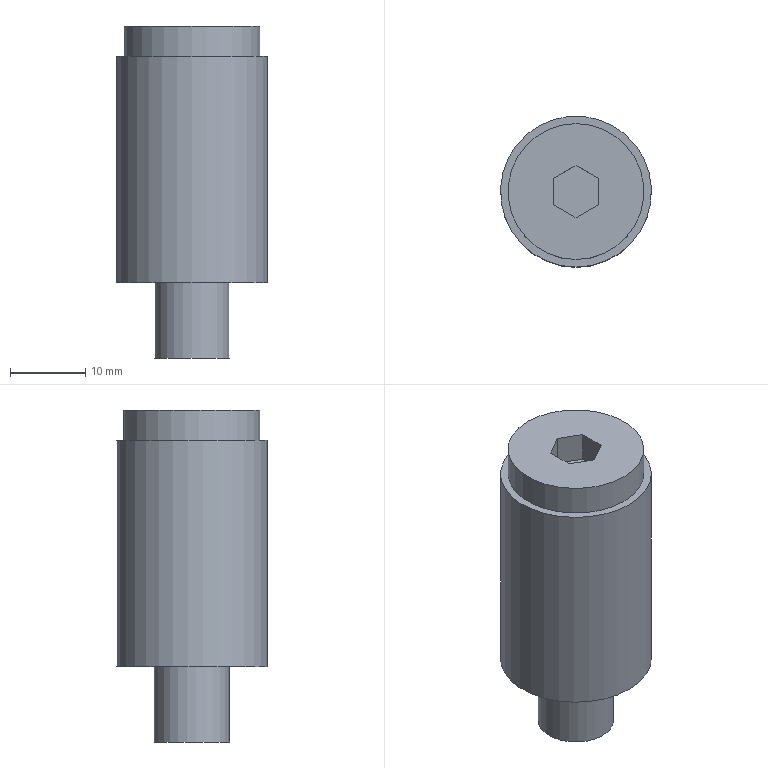Part | STEP file | 1_id570_xmt_txt | 1 solid | 17 faces | box 20 x 20 x 44 mm | volume 10770 mm3 | plane 12 | cylinder 4 | cone 1 | commonest cylinder face diameters 10 x1 11 x1 18 x1 20 x1
STEP:
#1=CARTESIAN_POINT('',(165.,186.,52.));
#2=VERTEX_POINT('',#1);
#3=CARTESIAN_POINT('',(165.,195.,52.));
#4=DIRECTION('',(0.,0.,1.));
#5=DIRECTION('',(0.,-1.,0.));
#6=AXIS2_PLACEMENT_3D('',#3,#4,#5);
#7=CIRCLE('',#6,9.);
#8=EDGE_CURVE('',#2,#2,#7,.T.);
#9=ORIENTED_EDGE('',*,*,#8,.F.);
#10=EDGE_LOOP('',(#9));
#11=FACE_BOUND('',#10,.T.);
#12=CARTESIAN_POINT('',(165.,186.,48.));
#13=VERTEX_POINT('',#12);
#14=CARTESIAN_POINT('',(165.,195.,48.));
#15=DIRECTION('',(0.,0.,-1.));
#16=DIRECTION('',(0.,-1.,0.));
#17=AXIS2_PLACEMENT_3D('',#14,#15,#16);
#18=CIRCLE('',#17,9.);
#19=EDGE_CURVE('',#13,#13,#18,.T.);
#20=ORIENTED_EDGE('',*,*,#19,.F.);
#21=EDGE_LOOP('',(#20));
#22=FACE_BOUND('',#21,.T.);
#23=CARTESIAN_POINT('',(165.,195.,50.));
#24=DIRECTION('',(0.,0.,-1.));
#25=DIRECTION('',(0.,1.,0.));
#26=AXIS2_PLACEMENT_3D('',#23,#24,#25);
#27=CYLINDRICAL_SURFACE('',#26,9.);
#28=ADVANCED_FACE('',(#11,#22),#27,.T.);
#29=CARTESIAN_POINT('',(165.,189.6,48.));
#30=VERTEX_POINT('',#29);
#31=CARTESIAN_POINT('',(165.,195.,48.));
#32=DIRECTION('',(0.,0.,1.));
#33=DIRECTION('',(0.,-1.,0.));
#34=AXIS2_PLACEMENT_3D('',#31,#32,#33);
#35=CIRCLE('',#34,5.4);
#36=EDGE_CURVE('',#30,#30,#35,.T.);
#37=ORIENTED_EDGE('',*,*,#36,.F.);
#38=EDGE_LOOP('',(#37));
#39=FACE_BOUND('',#38,.T.);
#40=CARTESIAN_POINT('',(165.,190.,23.));
#41=VERTEX_POINT('',#40);
#42=CARTESIAN_POINT('',(165.,195.,23.));
#43=DIRECTION('',(0.,0.,-1.));
#44=DIRECTION('',(0.,-1.,0.));
#45=AXIS2_PLACEMENT_3D('',#42,#43,#44);
#46=CIRCLE('',#45,5.);
#47=EDGE_CURVE('',#41,#41,#46,.T.);
#48=ORIENTED_EDGE('',*,*,#47,.F.);
#49=EDGE_LOOP('',(#48));
#50=FACE_BOUND('',#49,.T.);
#51=CARTESIAN_POINT('',(165.,195.,35.5));
#52=DIRECTION('',(0.,0.,1.));
#53=DIRECTION('',(0.,1.,0.));
#54=AXIS2_PLACEMENT_3D('',#51,#52,#53);
#55=CONICAL_SURFACE('',#54,5.2,0.9167);
#56=ADVANCED_FACE('',(#39,#50),#55,.T.);
#57=ORIENTED_EDGE('',*,*,#47,.T.);
#58=EDGE_LOOP('',(#57));
#59=FACE_BOUND('',#58,.T.);
#60=CARTESIAN_POINT('',(165.,190.,8.));
#61=VERTEX_POINT('',#60);
#62=CARTESIAN_POINT('',(165.,195.,8.));
#63=DIRECTION('',(0.,0.,-1.));
#64=DIRECTION('',(0.,-1.,0.));
#65=AXIS2_PLACEMENT_3D('',#62,#63,#64);
#66=CIRCLE('',#65,5.);
#67=EDGE_CURVE('',#61,#61,#66,.T.);
#68=ORIENTED_EDGE('',*,*,#67,.F.);
#69=EDGE_LOOP('',(#68));
#70=FACE_BOUND('',#69,.T.);
#71=CARTESIAN_POINT('',(165.,195.,15.5));
#72=DIRECTION('',(0.,0.,-1.));
#73=DIRECTION('',(0.,1.,0.));
#74=AXIS2_PLACEMENT_3D('',#71,#72,#73);
#75=CYLINDRICAL_SURFACE('',#74,5.);
#76=ADVANCED_FACE('',(#59,#70),#75,.T.);
#77=CARTESIAN_POINT('',(165.,185.,48.));
#78=VERTEX_POINT('',#77);
#79=CARTESIAN_POINT('',(165.,195.,48.));
#80=DIRECTION('',(0.,0.,1.));
#81=DIRECTION('',(0.,-1.,0.));
#82=AXIS2_PLACEMENT_3D('',#79,#80,#81);
#83=CIRCLE('',#82,10.);
#84=EDGE_CURVE('',#78,#78,#83,.T.);
#85=ORIENTED_EDGE('',*,*,#84,.F.);
#86=EDGE_LOOP('',(#85));
#87=FACE_BOUND('',#86,.T.);
#88=CARTESIAN_POINT('',(165.,185.,18.));
#89=VERTEX_POINT('',#88);
#90=CARTESIAN_POINT('',(165.,195.,18.));
#91=DIRECTION('',(0.,0.,-1.));
#92=DIRECTION('',(0.,-1.,0.));
#93=AXIS2_PLACEMENT_3D('',#90,#91,#92);
#94=CIRCLE('',#93,10.);
#95=EDGE_CURVE('',#89,#89,#94,.T.);
#96=ORIENTED_EDGE('',*,*,#95,.F.);
#97=EDGE_LOOP('',(#96));
#98=FACE_BOUND('',#97,.T.);
#99=CARTESIAN_POINT('',(165.,195.,33.));
#100=DIRECTION('',(0.,0.,-1.));
#101=DIRECTION('',(0.,1.,0.));
#102=AXIS2_PLACEMENT_3D('',#99,#100,#101);
#103=CYLINDRICAL_SURFACE('',#102,10.);
#104=ADVANCED_FACE('',(#87,#98),#103,.T.);
#105=CARTESIAN_POINT('',(165.,189.5,18.));
#106=VERTEX_POINT('',#105);
#107=CARTESIAN_POINT('',(165.,195.,18.));
#108=DIRECTION('',(0.,0.,1.));
#109=DIRECTION('',(0.,-1.,0.));
#110=AXIS2_PLACEMENT_3D('',#107,#108,#109);
#111=CIRCLE('',#110,5.5);
#112=EDGE_CURVE('',#106,#106,#111,.T.);
#113=ORIENTED_EDGE('',*,*,#112,.F.);
#114=EDGE_LOOP('',(#113));
#115=FACE_BOUND('',#114,.T.);
#116=CARTESIAN_POINT('',(165.,189.5,48.));
#117=VERTEX_POINT('',#116);
#118=CARTESIAN_POINT('',(165.,195.,48.));
#119=DIRECTION('',(0.,0.,-1.));
#120=DIRECTION('',(0.,-1.,0.));
#121=AXIS2_PLACEMENT_3D('',#118,#119,#120);
#122=CIRCLE('',#121,5.5);
#123=EDGE_CURVE('',#117,#117,#122,.T.);
#124=ORIENTED_EDGE('',*,*,#123,.F.);
#125=EDGE_LOOP('',(#124));
#126=FACE_BOUND('',#125,.T.);
#127=CARTESIAN_POINT('',(165.,195.,33.));
#128=DIRECTION('',(0.,0.,-1.));
#129=DIRECTION('',(0.,1.,0.));
#130=AXIS2_PLACEMENT_3D('',#127,#128,#129);
#131=CYLINDRICAL_SURFACE('',#130,5.5);
#132=ADVANCED_FACE('',(#115,#126),#131,.F.);
#133=ORIENTED_EDGE('',*,*,#84,.T.);
#134=EDGE_LOOP('',(#133));
#135=FACE_BOUND('',#134,.T.);
#136=ORIENTED_EDGE('',*,*,#19,.T.);
#137=EDGE_LOOP('',(#136));
#138=FACE_BOUND('',#137,.T.);
#139=CARTESIAN_POINT('',(165.,195.,48.));
#140=DIRECTION('',(0.,0.,1.));
#141=DIRECTION('',(0.,-1.,0.));
#142=AXIS2_PLACEMENT_3D('',#139,#140,#141);
#143=PLANE('',#142);
#144=ADVANCED_FACE('',(#135,#138),#143,.T.);
#145=ORIENTED_EDGE('',*,*,#112,.T.);
#146=EDGE_LOOP('',(#145));
#147=FACE_BOUND('',#146,.T.);
#148=ORIENTED_EDGE('',*,*,#95,.T.);
#149=EDGE_LOOP('',(#148));
#150=FACE_BOUND('',#149,.T.);
#151=CARTESIAN_POINT('',(165.,195.,18.));
#152=DIRECTION('',(0.,0.,-1.));
#153=DIRECTION('',(0.,1.,0.));
#154=AXIS2_PLACEMENT_3D('',#151,#152,#153);
#155=PLANE('',#154);
#156=ADVANCED_FACE('',(#147,#150),#155,.T.);
#157=CARTESIAN_POINT('',(162.,196.732,48.));
#158=VERTEX_POINT('',#157);
#159=CARTESIAN_POINT('',(162.,193.268,48.));
#160=VERTEX_POINT('',#159);
#161=CARTESIAN_POINT('',(162.,196.732,48.));
#162=DIRECTION('',(0.,-1.,0.));
#163=VECTOR('',#162,1.);
#164=LINE('',#161,#163);
#165=EDGE_CURVE('',#158,#160,#164,.T.);
#166=ORIENTED_EDGE('',*,*,#165,.F.);
#167=CARTESIAN_POINT('',(162.,196.732,52.));
#168=VERTEX_POINT('',#167);
#169=CARTESIAN_POINT('',(162.,196.732,52.));
#170=DIRECTION('',(0.,0.,-1.));
#171=VECTOR('',#170,1.);
#172=LINE('',#169,#171);
#173=EDGE_CURVE('',#168,#158,#172,.T.);
#174=ORIENTED_EDGE('',*,*,#173,.F.);
#175=CARTESIAN_POINT('',(162.,193.268,52.));
#176=VERTEX_POINT('',#175);
#177=CARTESIAN_POINT('',(162.,195.,52.));
#178=DIRECTION('',(0.,1.,0.));
#179=VECTOR('',#178,1.);
#180=LINE('',#177,#179);
#181=EDGE_CURVE('',#176,#168,#180,.T.);
#182=ORIENTED_EDGE('',*,*,#181,.F.);
#183=CARTESIAN_POINT('',(162.,193.268,52.));
#184=DIRECTION('',(0.,0.,-1.));
#185=VECTOR('',#184,1.);
#186=LINE('',#183,#185);
#187=EDGE_CURVE('',#176,#160,#186,.T.);
#188=ORIENTED_EDGE('',*,*,#187,.T.);
#189=EDGE_LOOP('',(#166,#174,#182,#188));
#190=FACE_OUTER_BOUND('',#189,.T.);
#191=CARTESIAN_POINT('',(162.,195.,52.));
#192=DIRECTION('',(-1.,0.,0.));
#193=DIRECTION('',(0.,-1.,0.));
#194=AXIS2_PLACEMENT_3D('',#191,#192,#193);
#195=PLANE('',#194);
#196=ADVANCED_FACE('',(#190),#195,.F.);
#197=CARTESIAN_POINT('',(165.,191.536,48.));
#198=VERTEX_POINT('',#197);
#199=CARTESIAN_POINT('',(162.,193.268,48.));
#200=DIRECTION('',(0.866,-0.5,0.));
#201=VECTOR('',#200,1.);
#202=LINE('',#199,#201);
#203=EDGE_CURVE('',#160,#198,#202,.T.);
#204=ORIENTED_EDGE('',*,*,#203,.F.);
#205=ORIENTED_EDGE('',*,*,#187,.F.);
#206=CARTESIAN_POINT('',(165.,191.536,52.));
#207=VERTEX_POINT('',#206);
#208=CARTESIAN_POINT('',(163.5,192.402,52.));
#209=DIRECTION('',(-0.866,0.5,0.));
#210=VECTOR('',#209,1.);
#211=LINE('',#208,#210);
#212=EDGE_CURVE('',#207,#176,#211,.T.);
#213=ORIENTED_EDGE('',*,*,#212,.F.);
#214=CARTESIAN_POINT('',(165.,191.536,52.));
#215=DIRECTION('',(0.,0.,-1.));
#216=VECTOR('',#215,1.);
#217=LINE('',#214,#216);
#218=EDGE_CURVE('',#207,#198,#217,.T.);
#219=ORIENTED_EDGE('',*,*,#218,.T.);
#220=EDGE_LOOP('',(#204,#205,#213,#219));
#221=FACE_OUTER_BOUND('',#220,.T.);
#222=CARTESIAN_POINT('',(163.5,192.402,52.));
#223=DIRECTION('',(-0.5,-0.866,0.));
#224=DIRECTION('',(0.866,-0.5,0.));
#225=AXIS2_PLACEMENT_3D('',#222,#223,#224);
#226=PLANE('',#225);
#227=ADVANCED_FACE('',(#221),#226,.F.);
#228=CARTESIAN_POINT('',(168.,193.268,48.));
#229=VERTEX_POINT('',#228);
#230=CARTESIAN_POINT('',(165.,191.536,48.));
#231=DIRECTION('',(0.866,0.5,0.));
#232=VECTOR('',#231,1.);
#233=LINE('',#230,#232);
#234=EDGE_CURVE('',#198,#229,#233,.T.);
#235=ORIENTED_EDGE('',*,*,#234,.F.);
#236=ORIENTED_EDGE('',*,*,#218,.F.);
#237=CARTESIAN_POINT('',(168.,193.268,52.));
#238=VERTEX_POINT('',#237);
#239=CARTESIAN_POINT('',(166.5,192.402,52.));
#240=DIRECTION('',(-0.866,-0.5,0.));
#241=VECTOR('',#240,1.);
#242=LINE('',#239,#241);
#243=EDGE_CURVE('',#238,#207,#242,.T.);
#244=ORIENTED_EDGE('',*,*,#243,.F.);
#245=CARTESIAN_POINT('',(168.,193.268,52.));
#246=DIRECTION('',(0.,0.,-1.));
#247=VECTOR('',#246,1.);
#248=LINE('',#245,#247);
#249=EDGE_CURVE('',#238,#229,#248,.T.);
#250=ORIENTED_EDGE('',*,*,#249,.T.);
#251=EDGE_LOOP('',(#235,#236,#244,#250));
#252=FACE_OUTER_BOUND('',#251,.T.);
#253=CARTESIAN_POINT('',(166.5,192.402,52.));
#254=DIRECTION('',(0.5,-0.866,0.));
#255=DIRECTION('',(0.866,0.5,0.));
#256=AXIS2_PLACEMENT_3D('',#253,#254,#255);
#257=PLANE('',#256);
#258=ADVANCED_FACE('',(#252),#257,.F.);
#259=CARTESIAN_POINT('',(168.,196.732,48.));
#260=VERTEX_POINT('',#259);
#261=CARTESIAN_POINT('',(168.,193.268,48.));
#262=DIRECTION('',(0.,1.,0.));
#263=VECTOR('',#262,1.);
#264=LINE('',#261,#263);
#265=EDGE_CURVE('',#229,#260,#264,.T.);
#266=ORIENTED_EDGE('',*,*,#265,.F.);
#267=ORIENTED_EDGE('',*,*,#249,.F.);
#268=CARTESIAN_POINT('',(168.,196.732,52.));
#269=VERTEX_POINT('',#268);
#270=CARTESIAN_POINT('',(168.,195.,52.));
#271=DIRECTION('',(0.,-1.,0.));
#272=VECTOR('',#271,1.);
#273=LINE('',#270,#272);
#274=EDGE_CURVE('',#269,#238,#273,.T.);
#275=ORIENTED_EDGE('',*,*,#274,.F.);
#276=CARTESIAN_POINT('',(168.,196.732,52.));
#277=DIRECTION('',(0.,0.,-1.));
#278=VECTOR('',#277,1.);
#279=LINE('',#276,#278);
#280=EDGE_CURVE('',#269,#260,#279,.T.);
#281=ORIENTED_EDGE('',*,*,#280,.T.);
#282=EDGE_LOOP('',(#266,#267,#275,#281));
#283=FACE_OUTER_BOUND('',#282,.T.);
#284=CARTESIAN_POINT('',(168.,195.,52.));
#285=DIRECTION('',(1.,0.,0.));
#286=DIRECTION('',(0.,1.,0.));
#287=AXIS2_PLACEMENT_3D('',#284,#285,#286);
#288=PLANE('',#287);
#289=ADVANCED_FACE('',(#283),#288,.F.);
#290=CARTESIAN_POINT('',(165.,198.464,48.));
#291=VERTEX_POINT('',#290);
#292=CARTESIAN_POINT('',(168.,196.732,48.));
#293=DIRECTION('',(-0.866,0.5,0.));
#294=VECTOR('',#293,1.);
#295=LINE('',#292,#294);
#296=EDGE_CURVE('',#260,#291,#295,.T.);
#297=ORIENTED_EDGE('',*,*,#296,.F.);
#298=ORIENTED_EDGE('',*,*,#280,.F.);
#299=CARTESIAN_POINT('',(165.,198.464,52.));
#300=VERTEX_POINT('',#299);
#301=CARTESIAN_POINT('',(166.5,197.598,52.));
#302=DIRECTION('',(0.866,-0.5,0.));
#303=VECTOR('',#302,1.);
#304=LINE('',#301,#303);
#305=EDGE_CURVE('',#300,#269,#304,.T.);
#306=ORIENTED_EDGE('',*,*,#305,.F.);
#307=CARTESIAN_POINT('',(165.,198.464,52.));
#308=DIRECTION('',(0.,0.,-1.));
#309=VECTOR('',#308,1.);
#310=LINE('',#307,#309);
#311=EDGE_CURVE('',#300,#291,#310,.T.);
#312=ORIENTED_EDGE('',*,*,#311,.T.);
#313=EDGE_LOOP('',(#297,#298,#306,#312));
#314=FACE_OUTER_BOUND('',#313,.T.);
#315=CARTESIAN_POINT('',(166.5,197.598,52.));
#316=DIRECTION('',(0.5,0.866,0.));
#317=DIRECTION('',(-0.866,0.5,0.));
#318=AXIS2_PLACEMENT_3D('',#315,#316,#317);
#319=PLANE('',#318);
#320=ADVANCED_FACE('',(#314),#319,.F.);
#321=CARTESIAN_POINT('',(165.,198.464,48.));
#322=DIRECTION('',(-0.866,-0.5,0.));
#323=VECTOR('',#322,1.);
#324=LINE('',#321,#323);
#325=EDGE_CURVE('',#291,#158,#324,.T.);
#326=ORIENTED_EDGE('',*,*,#325,.F.);
#327=ORIENTED_EDGE('',*,*,#311,.F.);
#328=CARTESIAN_POINT('',(163.5,197.598,52.));
#329=DIRECTION('',(0.866,0.5,0.));
#330=VECTOR('',#329,1.);
#331=LINE('',#328,#330);
#332=EDGE_CURVE('',#168,#300,#331,.T.);
#333=ORIENTED_EDGE('',*,*,#332,.F.);
#334=ORIENTED_EDGE('',*,*,#173,.T.);
#335=EDGE_LOOP('',(#326,#327,#333,#334));
#336=FACE_OUTER_BOUND('',#335,.T.);
#337=CARTESIAN_POINT('',(163.5,197.598,52.));
#338=DIRECTION('',(-0.5,0.866,0.));
#339=DIRECTION('',(-0.866,-0.5,0.));
#340=AXIS2_PLACEMENT_3D('',#337,#338,#339);
#341=PLANE('',#340);
#342=ADVANCED_FACE('',(#336),#341,.F.);
#343=ORIENTED_EDGE('',*,*,#165,.T.);
#344=ORIENTED_EDGE('',*,*,#203,.T.);
#345=ORIENTED_EDGE('',*,*,#234,.T.);
#346=ORIENTED_EDGE('',*,*,#265,.T.);
#347=ORIENTED_EDGE('',*,*,#296,.T.);
#348=ORIENTED_EDGE('',*,*,#325,.T.);
#349=EDGE_LOOP('',(#343,#344,#345,#346,#347,#348));
#350=FACE_OUTER_BOUND('',#349,.T.);
#351=CARTESIAN_POINT('',(165.,195.,48.));
#352=DIRECTION('',(0.,0.,-1.));
#353=DIRECTION('',(0.,1.,0.));
#354=AXIS2_PLACEMENT_3D('',#351,#352,#353);
#355=PLANE('',#354);
#356=ADVANCED_FACE('',(#350),#355,.F.);
#357=ORIENTED_EDGE('',*,*,#67,.T.);
#358=EDGE_LOOP('',(#357));
#359=FACE_OUTER_BOUND('',#358,.T.);
#360=CARTESIAN_POINT('',(165.,195.,8.));
#361=DIRECTION('',(0.,0.,-1.));
#362=DIRECTION('',(0.,1.,0.));
#363=AXIS2_PLACEMENT_3D('',#360,#361,#362);
#364=PLANE('',#363);
#365=ADVANCED_FACE('',(#359),#364,.T.);
#366=ORIENTED_EDGE('',*,*,#181,.T.);
#367=ORIENTED_EDGE('',*,*,#332,.T.);
#368=ORIENTED_EDGE('',*,*,#305,.T.);
#369=ORIENTED_EDGE('',*,*,#274,.T.);
#370=ORIENTED_EDGE('',*,*,#243,.T.);
#371=ORIENTED_EDGE('',*,*,#212,.T.);
#372=EDGE_LOOP('',(#366,#367,#368,#369,#370,#371));
#373=FACE_BOUND('',#372,.T.);
#374=ORIENTED_EDGE('',*,*,#8,.T.);
#375=EDGE_LOOP('',(#374));
#376=FACE_BOUND('',#375,.T.);
#377=CARTESIAN_POINT('',(165.,195.,52.));
#378=DIRECTION('',(0.,0.,1.));
#379=DIRECTION('',(0.,-1.,0.));
#380=AXIS2_PLACEMENT_3D('',#377,#378,#379);
#381=PLANE('',#380);
#382=ADVANCED_FACE('',(#373,#376),#381,.T.);
#383=ORIENTED_EDGE('',*,*,#123,.T.);
#384=EDGE_LOOP('',(#383));
#385=FACE_BOUND('',#384,.T.);
#386=ORIENTED_EDGE('',*,*,#36,.T.);
#387=EDGE_LOOP('',(#386));
#388=FACE_BOUND('',#387,.T.);
#389=CARTESIAN_POINT('',(165.,195.,48.));
#390=DIRECTION('',(0.,0.,-1.));
#391=DIRECTION('',(0.,1.,0.));
#392=AXIS2_PLACEMENT_3D('',#389,#390,#391);
#393=PLANE('',#392);
#394=ADVANCED_FACE('',(#385,#388),#393,.T.);
#395=CLOSED_SHELL('',(#28,#56,#76,#104,#132,#144,#156,#196,#227,#258,#289,#320,#342,#356,#365,#382,#394));
#396=MANIFOLD_SOLID_BREP('',#395);
#397=(LENGTH_UNIT()NAMED_UNIT(*)SI_UNIT(.MILLI.,.METRE.));
#398=UNCERTAINTY_MEASURE_WITH_UNIT(LENGTH_MEASURE(0.00002),#397,'','');
#399=(NAMED_UNIT(*)PLANE_ANGLE_UNIT()SI_UNIT($,.RADIAN.));
#400=PLANE_ANGLE_MEASURE_WITH_UNIT(PLANE_ANGLE_MEASURE(0.01745),#399);
#401=DIMENSIONAL_EXPONENTS(0.,0.,0.,0.,0.,0.,0.);
#402=(CONVERSION_BASED_UNIT('DEGREE',#400)NAMED_UNIT(#401)PLANE_ANGLE_UNIT());
#403=(NAMED_UNIT(*)SI_UNIT($,.STERADIAN.)SOLID_ANGLE_UNIT());
#404=(GEOMETRIC_REPRESENTATION_CONTEXT(3)GLOBAL_UNCERTAINTY_ASSIGNED_CONTEXT((#398))GLOBAL_UNIT_ASSIGNED_CONTEXT((#397,#402,#403))REPRESENTATION_CONTEXT('',''));
#405=ADVANCED_BREP_SHAPE_REPRESENTATION('',(#396),#404);